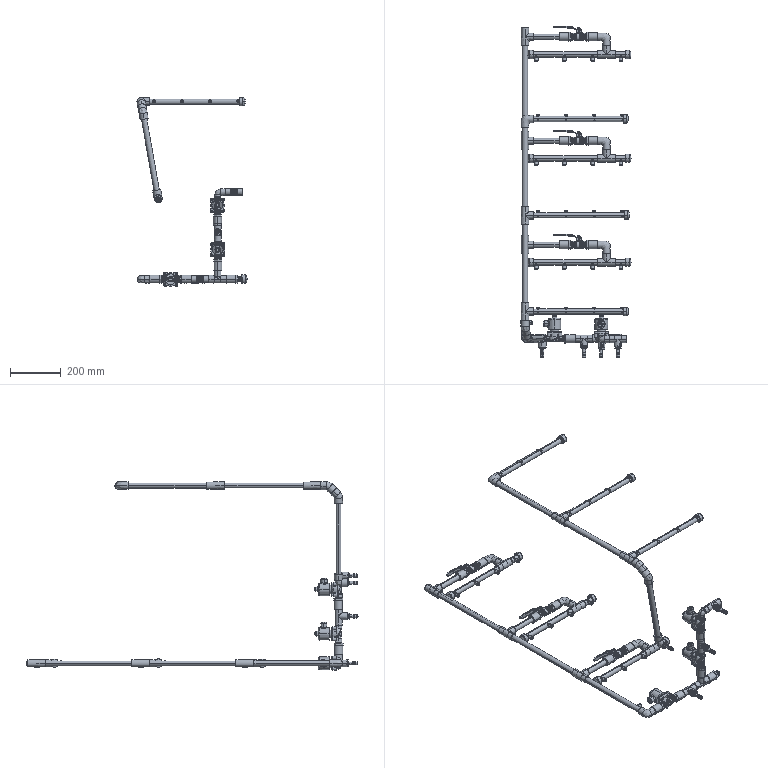Part | SolidWorks | 144 solids | 5805 faces | volume 2759072 mm3 | cylinder 1702 | plane 1404 | cone 1199 | spline 1057 | torus 287 | sphere 156 | commonest cylinder face diameters 0.635 x186 13.868 x121 19.583 x120 8 x112 18.5 x111 10 x98